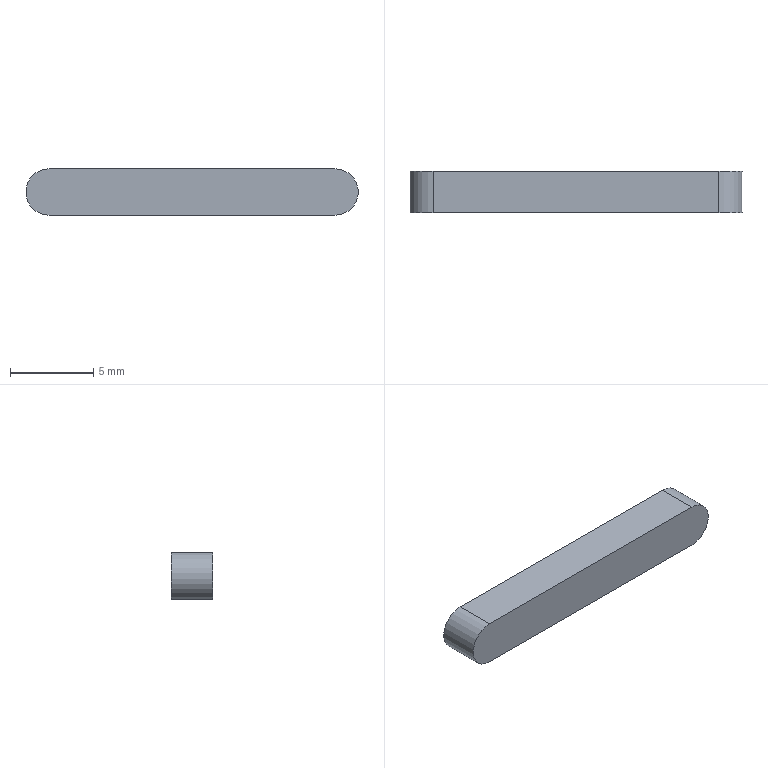Part | SolidWorks | features Extrusion 1 | 1 solid | 6 faces | box 20 x 2.5 x 2.8 mm | volume 135.794 mm3 | plane 4 | cylinder 2 | commonest cylinder face diameters 2.8 x2
STEP:
#1=CARTESIAN_POINT('',(-8.6,0.,-1.4));
#2=VERTEX_POINT('',#1);
#3=CARTESIAN_POINT('',(-8.6,0.,1.4));
#4=VERTEX_POINT('',#3);
#5=CARTESIAN_POINT('',(-8.6,0.,0.));
#6=DIRECTION('',(0.,1.,0.));
#7=DIRECTION('',(0.,0.,-1.));
#8=AXIS2_PLACEMENT_3D('',#5,#6,#7);
#9=CIRCLE('',#8,1.4);
#10=EDGE_CURVE('',#2,#4,#9,.T.);
#11=ORIENTED_EDGE('',*,*,#10,.T.);
#12=CARTESIAN_POINT('',(-8.6,2.5,1.4));
#13=VERTEX_POINT('',#12);
#14=CARTESIAN_POINT('',(-8.6,2.5,1.4));
#15=DIRECTION('',(0.,-1.,0.));
#16=VECTOR('',#15,1000.);
#17=LINE('',#14,#16);
#18=EDGE_CURVE('',#13,#4,#17,.T.);
#19=ORIENTED_EDGE('',*,*,#18,.F.);
#20=CARTESIAN_POINT('',(-8.6,2.5,-1.4));
#21=VERTEX_POINT('',#20);
#22=CARTESIAN_POINT('',(-8.6,2.5,0.));
#23=DIRECTION('',(0.,1.,0.));
#24=DIRECTION('',(0.,0.,-1.));
#25=AXIS2_PLACEMENT_3D('',#22,#23,#24);
#26=CIRCLE('',#25,1.4);
#27=EDGE_CURVE('',#21,#13,#26,.T.);
#28=ORIENTED_EDGE('',*,*,#27,.F.);
#29=CARTESIAN_POINT('',(-8.6,2.5,-1.4));
#30=DIRECTION('',(0.,-1.,0.));
#31=VECTOR('',#30,1000.);
#32=LINE('',#29,#31);
#33=EDGE_CURVE('',#21,#2,#32,.T.);
#34=ORIENTED_EDGE('',*,*,#33,.T.);
#35=EDGE_LOOP('',(#11,#19,#28,#34));
#36=FACE_OUTER_BOUND('',#35,.T.);
#37=CARTESIAN_POINT('',(-8.6,2.5,0.));
#38=DIRECTION('',(0.,-1.,0.));
#39=DIRECTION('',(0.,0.,-1.));
#40=AXIS2_PLACEMENT_3D('',#37,#38,#39);
#41=CYLINDRICAL_SURFACE('',#40,1.4);
#42=ADVANCED_FACE('',(#36),#41,.T.);
#43=CARTESIAN_POINT('',(8.6,0.,1.4));
#44=VERTEX_POINT('',#43);
#45=CARTESIAN_POINT('',(8.6,0.,1.4));
#46=DIRECTION('',(1.,0.,0.));
#47=VECTOR('',#46,1000.);
#48=LINE('',#45,#47);
#49=EDGE_CURVE('',#4,#44,#48,.T.);
#50=ORIENTED_EDGE('',*,*,#49,.T.);
#51=CARTESIAN_POINT('',(8.6,2.5,1.4));
#52=VERTEX_POINT('',#51);
#53=CARTESIAN_POINT('',(8.6,2.5,1.4));
#54=DIRECTION('',(0.,-1.,0.));
#55=VECTOR('',#54,1000.);
#56=LINE('',#53,#55);
#57=EDGE_CURVE('',#52,#44,#56,.T.);
#58=ORIENTED_EDGE('',*,*,#57,.F.);
#59=CARTESIAN_POINT('',(8.6,2.5,1.4));
#60=DIRECTION('',(1.,0.,0.));
#61=VECTOR('',#60,1000.);
#62=LINE('',#59,#61);
#63=EDGE_CURVE('',#13,#52,#62,.T.);
#64=ORIENTED_EDGE('',*,*,#63,.F.);
#65=ORIENTED_EDGE('',*,*,#18,.T.);
#66=EDGE_LOOP('',(#50,#58,#64,#65));
#67=FACE_OUTER_BOUND('',#66,.T.);
#68=CARTESIAN_POINT('',(8.6,2.5,1.4));
#69=DIRECTION('',(0.,0.,-1.));
#70=DIRECTION('',(-1.,0.,0.));
#71=AXIS2_PLACEMENT_3D('',#68,#69,#70);
#72=PLANE('',#71);
#73=ADVANCED_FACE('',(#67),#72,.F.);
#74=CARTESIAN_POINT('',(8.6,0.,-1.4));
#75=VERTEX_POINT('',#74);
#76=CARTESIAN_POINT('',(8.6,0.,0.));
#77=DIRECTION('',(0.,1.,0.));
#78=DIRECTION('',(0.,0.,-1.));
#79=AXIS2_PLACEMENT_3D('',#76,#77,#78);
#80=CIRCLE('',#79,1.4);
#81=EDGE_CURVE('',#44,#75,#80,.T.);
#82=ORIENTED_EDGE('',*,*,#81,.T.);
#83=CARTESIAN_POINT('',(8.6,2.5,-1.4));
#84=VERTEX_POINT('',#83);
#85=CARTESIAN_POINT('',(8.6,2.5,-1.4));
#86=DIRECTION('',(0.,-1.,0.));
#87=VECTOR('',#86,1000.);
#88=LINE('',#85,#87);
#89=EDGE_CURVE('',#84,#75,#88,.T.);
#90=ORIENTED_EDGE('',*,*,#89,.F.);
#91=CARTESIAN_POINT('',(8.6,2.5,0.));
#92=DIRECTION('',(0.,1.,0.));
#93=DIRECTION('',(0.,0.,-1.));
#94=AXIS2_PLACEMENT_3D('',#91,#92,#93);
#95=CIRCLE('',#94,1.4);
#96=EDGE_CURVE('',#52,#84,#95,.T.);
#97=ORIENTED_EDGE('',*,*,#96,.F.);
#98=ORIENTED_EDGE('',*,*,#57,.T.);
#99=EDGE_LOOP('',(#82,#90,#97,#98));
#100=FACE_OUTER_BOUND('',#99,.T.);
#101=CARTESIAN_POINT('',(8.6,2.5,0.));
#102=DIRECTION('',(0.,-1.,0.));
#103=DIRECTION('',(0.,0.,-1.));
#104=AXIS2_PLACEMENT_3D('',#101,#102,#103);
#105=CYLINDRICAL_SURFACE('',#104,1.4);
#106=ADVANCED_FACE('',(#100),#105,.T.);
#107=CARTESIAN_POINT('',(-8.6,0.,-1.4));
#108=DIRECTION('',(-1.,0.,0.));
#109=VECTOR('',#108,1000.);
#110=LINE('',#107,#109);
#111=EDGE_CURVE('',#75,#2,#110,.T.);
#112=ORIENTED_EDGE('',*,*,#111,.T.);
#113=ORIENTED_EDGE('',*,*,#33,.F.);
#114=CARTESIAN_POINT('',(-8.6,2.5,-1.4));
#115=DIRECTION('',(-1.,0.,0.));
#116=VECTOR('',#115,1000.);
#117=LINE('',#114,#116);
#118=EDGE_CURVE('',#84,#21,#117,.T.);
#119=ORIENTED_EDGE('',*,*,#118,.F.);
#120=ORIENTED_EDGE('',*,*,#89,.T.);
#121=EDGE_LOOP('',(#112,#113,#119,#120));
#122=FACE_OUTER_BOUND('',#121,.T.);
#123=CARTESIAN_POINT('',(-8.6,2.5,-1.4));
#124=DIRECTION('',(0.,0.,1.));
#125=DIRECTION('',(1.,0.,0.));
#126=AXIS2_PLACEMENT_3D('',#123,#124,#125);
#127=PLANE('',#126);
#128=ADVANCED_FACE('',(#122),#127,.F.);
#129=ORIENTED_EDGE('',*,*,#27,.T.);
#130=ORIENTED_EDGE('',*,*,#63,.T.);
#131=ORIENTED_EDGE('',*,*,#96,.T.);
#132=ORIENTED_EDGE('',*,*,#118,.T.);
#133=EDGE_LOOP('',(#129,#130,#131,#132));
#134=FACE_OUTER_BOUND('',#133,.T.);
#135=CARTESIAN_POINT('',(-8.6,2.5,0.));
#136=DIRECTION('',(0.,-1.,0.));
#137=DIRECTION('',(0.,0.,-1.));
#138=AXIS2_PLACEMENT_3D('',#135,#136,#137);
#139=PLANE('',#138);
#140=ADVANCED_FACE('',(#134),#139,.F.);
#141=ORIENTED_EDGE('',*,*,#10,.F.);
#142=ORIENTED_EDGE('',*,*,#111,.F.);
#143=ORIENTED_EDGE('',*,*,#81,.F.);
#144=ORIENTED_EDGE('',*,*,#49,.F.);
#145=EDGE_LOOP('',(#141,#142,#143,#144));
#146=FACE_OUTER_BOUND('',#145,.T.);
#147=CARTESIAN_POINT('',(-8.6,0.,0.));
#148=DIRECTION('',(0.,-1.,0.));
#149=DIRECTION('',(0.,0.,-1.));
#150=AXIS2_PLACEMENT_3D('',#147,#148,#149);
#151=PLANE('',#150);
#152=ADVANCED_FACE('',(#146),#151,.T.);
#153=CLOSED_SHELL('',(#42,#73,#106,#128,#140,#152));
#154=MANIFOLD_SOLID_BREP('',#153);
#155=CARTESIAN_POINT('',(0.,0.,0.));
#156=DIRECTION('',(0.,0.,1.));
#157=DIRECTION('',(1.,0.,0.));
#158=AXIS2_PLACEMENT_3D('',#155,#156,#157);
#159=(LENGTH_UNIT()NAMED_UNIT(*)SI_UNIT(.MILLI.,.METRE.));
#160=UNCERTAINTY_MEASURE_WITH_UNIT(LENGTH_MEASURE(0.00001),#159,'','');
#161=(NAMED_UNIT(*)PLANE_ANGLE_UNIT()SI_UNIT($,.RADIAN.));
#162=(NAMED_UNIT(*)SI_UNIT($,.STERADIAN.)SOLID_ANGLE_UNIT());
#163=(GEOMETRIC_REPRESENTATION_CONTEXT(3)GLOBAL_UNCERTAINTY_ASSIGNED_CONTEXT((#160))GLOBAL_UNIT_ASSIGNED_CONTEXT((#159,#161,#162))REPRESENTATION_CONTEXT('',''));
#164=ADVANCED_BREP_SHAPE_REPRESENTATION('',(#154,#158),#163);